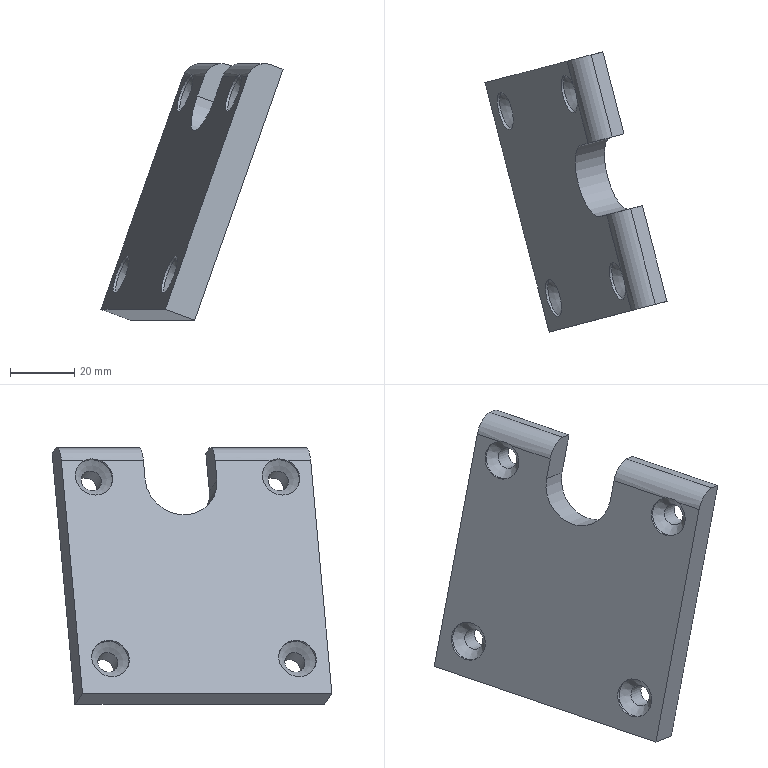Part | STEP file | 车灯-后视镜_id570_x_t | 1 solid | 24 faces | box 56.564 x 86.901 x 79.724 mm | volume 59028 mm3 | cylinder 11 | plane 9 | cone 4 | commonest cylinder face diameters 12 x6 6.5 x4 23 x1
STEP:
#1=CARTESIAN_POINT('',(-178.814,15.991,96.986));
#2=VERTEX_POINT('',#1);
#3=CARTESIAN_POINT('',(-176.662,16.547,103.094));
#4=VERTEX_POINT('',#3);
#5=CARTESIAN_POINT('',(-198.851,10.825,40.135));
#6=DIRECTION('',(0.3312,0.0854,0.9397));
#7=VECTOR('',#6,1.);
#8=LINE('',#5,#7);
#9=EDGE_CURVE('',#2,#4,#8,.T.);
#10=ORIENTED_EDGE('',*,*,#9,.T.);
#11=CARTESIAN_POINT('',(-169.215,18.467,106.68));
#12=VERTEX_POINT('',#11);
#13=CARTESIAN_POINT('',(-171.202,17.954,101.042));
#14=DIRECTION('',(-0.2497,0.9683,0.));
#15=DIRECTION('',(0.9683,0.2497,0.));
#16=AXIS2_PLACEMENT_3D('',#13,#14,#15);
#17=CIRCLE('',#16,6.);
#18=EDGE_CURVE('',#4,#12,#17,.T.);
#19=ORIENTED_EDGE('',*,*,#18,.T.);
#20=CARTESIAN_POINT('',(-165.575,19.405,105.312));
#21=VERTEX_POINT('',#20);
#22=CARTESIAN_POINT('',(-174.674,17.059,108.732));
#23=DIRECTION('',(0.9099,0.2346,-0.342));
#24=VECTOR('',#23,1.);
#25=LINE('',#22,#24);
#26=EDGE_CURVE('',#12,#21,#25,.T.);
#27=ORIENTED_EDGE('',*,*,#26,.T.);
#28=CARTESIAN_POINT('',(-169.715,18.338,93.566));
#29=VERTEX_POINT('',#28);
#30=CARTESIAN_POINT('',(-189.752,13.171,36.714));
#31=DIRECTION('',(0.3312,0.0854,0.9397));
#32=VECTOR('',#31,1.);
#33=LINE('',#30,#32);
#34=EDGE_CURVE('',#29,#21,#33,.T.);
#35=ORIENTED_EDGE('',*,*,#34,.F.);
#36=CARTESIAN_POINT('',(-157.987,21.362,89.158));
#37=DIRECTION('',(-0.9099,-0.2346,0.342));
#38=VECTOR('',#37,1.);
#39=LINE('',#36,#38);
#40=EDGE_CURVE('',#29,#2,#39,.T.);
#41=ORIENTED_EDGE('',*,*,#40,.T.);
#42=EDGE_LOOP('',(#10,#19,#27,#35,#41));
#43=FACE_OUTER_BOUND('',#42,.T.);
#44=CARTESIAN_POINT('',(-155.457,22.015,96.332));
#45=DIRECTION('',(0.2497,-0.9683,0.));
#46=DIRECTION('',(0.9683,0.2497,0.));
#47=AXIS2_PLACEMENT_3D('',#44,#45,#46);
#48=PLANE('',#47);
#49=ADVANCED_FACE('',(#43),#48,.F.);
#50=CARTESIAN_POINT('',(-161.554,-11.242,106.68));
#51=VERTEX_POINT('',#50);
#52=CARTESIAN_POINT('',(-157.914,-10.303,105.312));
#53=VERTEX_POINT('',#52);
#54=CARTESIAN_POINT('',(-167.013,-12.65,108.732));
#55=DIRECTION('',(0.9099,0.2346,-0.342));
#56=VECTOR('',#55,1.);
#57=LINE('',#54,#56);
#58=EDGE_CURVE('',#51,#53,#57,.T.);
#59=ORIENTED_EDGE('',*,*,#58,.F.);
#60=CARTESIAN_POINT('',(-169.001,-13.162,103.094));
#61=VERTEX_POINT('',#60);
#62=CARTESIAN_POINT('',(-163.541,-11.754,101.042));
#63=DIRECTION('',(0.2497,-0.9683,0.));
#64=DIRECTION('',(0.9683,0.2497,0.));
#65=AXIS2_PLACEMENT_3D('',#62,#63,#64);
#66=CIRCLE('',#65,6.);
#67=EDGE_CURVE('',#51,#61,#66,.T.);
#68=ORIENTED_EDGE('',*,*,#67,.T.);
#69=CARTESIAN_POINT('',(-194.502,-19.738,30.738));
#70=VERTEX_POINT('',#69);
#71=CARTESIAN_POINT('',(-178.886,-15.711,75.045));
#72=DIRECTION('',(-0.3312,-0.0854,-0.9397));
#73=VECTOR('',#72,1.);
#74=LINE('',#71,#73);
#75=EDGE_CURVE('',#61,#70,#74,.T.);
#76=ORIENTED_EDGE('',*,*,#75,.T.);
#77=CARTESIAN_POINT('',(-185.403,-17.392,27.318));
#78=VERTEX_POINT('',#77);
#79=CARTESIAN_POINT('',(-194.502,-19.738,30.738));
#80=DIRECTION('',(0.9099,0.2346,-0.342));
#81=VECTOR('',#80,1.);
#82=LINE('',#79,#81);
#83=EDGE_CURVE('',#70,#78,#82,.T.);
#84=ORIENTED_EDGE('',*,*,#83,.T.);
#85=CARTESIAN_POINT('',(-169.787,-13.365,71.625));
#86=DIRECTION('',(-0.3312,-0.0854,-0.9397));
#87=VECTOR('',#86,1.);
#88=LINE('',#85,#87);
#89=EDGE_CURVE('',#53,#78,#88,.T.);
#90=ORIENTED_EDGE('',*,*,#89,.F.);
#91=EDGE_LOOP('',(#59,#68,#76,#84,#90));
#92=FACE_OUTER_BOUND('',#91,.T.);
#93=CARTESIAN_POINT('',(-178.886,-15.711,75.045));
#94=DIRECTION('',(0.2497,-0.9683,0.));
#95=DIRECTION('',(0.9683,0.2497,0.));
#96=AXIS2_PLACEMENT_3D('',#93,#94,#95);
#97=PLANE('',#96);
#98=ADVANCED_FACE('',(#92),#97,.T.);
#99=CARTESIAN_POINT('',(-191.079,-9.073,47.161));
#100=VERTEX_POINT('',#99);
#101=CARTESIAN_POINT('',(-193.19,-9.073,41.544));
#102=DIRECTION('',(0.9099,0.2346,-0.342));
#103=DIRECTION('',(0.3518,0.,0.9361));
#104=AXIS2_PLACEMENT_3D('',#101,#102,#103);
#105=CIRCLE('',#104,6.);
#106=EDGE_CURVE('',#100,#100,#105,.T.);
#107=ORIENTED_EDGE('',*,*,#106,.T.);
#108=EDGE_LOOP('',(#107));
#109=FACE_BOUND('',#108,.T.);
#110=CARTESIAN_POINT('',(-206.061,49.027,47.161));
#111=VERTEX_POINT('',#110);
#112=CARTESIAN_POINT('',(-208.172,49.027,41.544));
#113=DIRECTION('',(0.9099,0.2346,-0.342));
#114=DIRECTION('',(0.3518,0.,0.9361));
#115=AXIS2_PLACEMENT_3D('',#112,#113,#114);
#116=CIRCLE('',#115,6.);
#117=EDGE_CURVE('',#111,#111,#116,.T.);
#118=ORIENTED_EDGE('',*,*,#117,.T.);
#119=EDGE_LOOP('',(#118));
#120=FACE_BOUND('',#119,.T.);
#121=CARTESIAN_POINT('',(-184.557,38.263,96.986));
#122=VERTEX_POINT('',#121);
#123=CARTESIAN_POINT('',(-182.405,38.818,103.094));
#124=VERTEX_POINT('',#123);
#125=CARTESIAN_POINT('',(-204.594,33.096,40.135));
#126=DIRECTION('',(0.3312,0.0854,0.9397));
#127=VECTOR('',#126,1.);
#128=LINE('',#125,#127);
#129=EDGE_CURVE('',#122,#124,#128,.T.);
#130=ORIENTED_EDGE('',*,*,#129,.T.);
#131=CARTESIAN_POINT('',(-185.881,52.298,103.094));
#132=VERTEX_POINT('',#131);
#133=CARTESIAN_POINT('',(-178.93,25.345,103.094));
#134=DIRECTION('',(-0.2497,0.9683,0.));
#135=VECTOR('',#134,1.);
#136=LINE('',#133,#135);
#137=EDGE_CURVE('',#124,#132,#136,.T.);
#138=ORIENTED_EDGE('',*,*,#137,.T.);
#139=CARTESIAN_POINT('',(-187.078,56.942,103.094));
#140=VERTEX_POINT('',#139);
#141=CARTESIAN_POINT('',(-188.301,54.151,97.926));
#142=DIRECTION('',(0.9099,0.2346,-0.342));
#143=DIRECTION('',(0.3518,0.,0.9361));
#144=AXIS2_PLACEMENT_3D('',#141,#142,#143);
#145=CIRCLE('',#144,6.);
#146=EDGE_CURVE('',#132,#140,#145,.T.);
#147=ORIENTED_EDGE('',*,*,#146,.T.);
#148=CARTESIAN_POINT('',(-188.976,64.304,103.094));
#149=VERTEX_POINT('',#148);
#150=CARTESIAN_POINT('',(-178.93,25.345,103.094));
#151=DIRECTION('',(-0.2497,0.9683,0.));
#152=VECTOR('',#151,1.);
#153=LINE('',#150,#152);
#154=EDGE_CURVE('',#140,#149,#153,.T.);
#155=ORIENTED_EDGE('',*,*,#154,.T.);
#156=CARTESIAN_POINT('',(-214.478,57.728,30.738));
#157=VERTEX_POINT('',#156);
#158=CARTESIAN_POINT('',(-198.862,61.754,75.045));
#159=DIRECTION('',(0.3312,0.0854,0.9397));
#160=VECTOR('',#159,1.);
#161=LINE('',#158,#160);
#162=EDGE_CURVE('',#157,#149,#161,.T.);
#163=ORIENTED_EDGE('',*,*,#162,.F.);
#164=CARTESIAN_POINT('',(-204.432,18.769,30.738));
#165=DIRECTION('',(-0.2497,0.9683,0.));
#166=VECTOR('',#165,1.);
#167=LINE('',#164,#166);
#168=EDGE_CURVE('',#70,#157,#167,.T.);
#169=ORIENTED_EDGE('',*,*,#168,.F.);
#170=ORIENTED_EDGE('',*,*,#75,.F.);
#171=CARTESIAN_POINT('',(-170.899,-5.801,103.094));
#172=VERTEX_POINT('',#171);
#173=CARTESIAN_POINT('',(-178.93,25.345,103.094));
#174=DIRECTION('',(-0.2497,0.9683,0.));
#175=VECTOR('',#174,1.);
#176=LINE('',#173,#175);
#177=EDGE_CURVE('',#61,#172,#176,.T.);
#178=ORIENTED_EDGE('',*,*,#177,.T.);
#179=CARTESIAN_POINT('',(-172.096,-1.157,103.094));
#180=VERTEX_POINT('',#179);
#181=CARTESIAN_POINT('',(-173.319,-3.949,97.926));
#182=DIRECTION('',(0.9099,0.2346,-0.342));
#183=DIRECTION('',(0.3518,0.,0.9361));
#184=AXIS2_PLACEMENT_3D('',#181,#182,#183);
#185=CIRCLE('',#184,6.);
#186=EDGE_CURVE('',#172,#180,#185,.T.);
#187=ORIENTED_EDGE('',*,*,#186,.T.);
#188=CARTESIAN_POINT('',(-178.93,25.345,103.094));
#189=DIRECTION('',(-0.2497,0.9683,0.));
#190=VECTOR('',#189,1.);
#191=LINE('',#188,#190);
#192=EDGE_CURVE('',#180,#4,#191,.T.);
#193=ORIENTED_EDGE('',*,*,#192,.T.);
#194=ORIENTED_EDGE('',*,*,#9,.F.);
#195=CARTESIAN_POINT('',(-181.686,27.127,96.986));
#196=DIRECTION('',(0.9099,0.2346,-0.342));
#197=DIRECTION('',(0.3518,0.,0.9361));
#198=AXIS2_PLACEMENT_3D('',#195,#196,#197);
#199=CIRCLE('',#198,11.5);
#200=EDGE_CURVE('',#2,#122,#199,.T.);
#201=ORIENTED_EDGE('',*,*,#200,.T.);
#202=EDGE_LOOP('',(#130,#138,#147,#155,#163,#169,#170,#178,#187,#193,#194,#201));
#203=FACE_BOUND('',#202,.T.);
#204=CARTESIAN_POINT('',(-201.12,19.623,40.135));
#205=DIRECTION('',(-0.9099,-0.2346,0.342));
#206=DIRECTION('',(0.3518,0.,0.9361));
#207=AXIS2_PLACEMENT_3D('',#204,#205,#206);
#208=PLANE('',#207);
#209=ADVANCED_FACE('',(#109,#120,#203),#208,.T.);
#210=CARTESIAN_POINT('',(-182.948,-6.726,41.166));
#211=VERTEX_POINT('',#210);
#212=CARTESIAN_POINT('',(-184.091,-6.726,38.124));
#213=DIRECTION('',(0.9099,0.2346,-0.342));
#214=DIRECTION('',(0.3518,0.,0.9361));
#215=AXIS2_PLACEMENT_3D('',#212,#213,#214);
#216=CIRCLE('',#215,3.25);
#217=EDGE_CURVE('',#211,#211,#216,.T.);
#218=ORIENTED_EDGE('',*,*,#217,.F.);
#219=EDGE_LOOP('',(#218));
#220=FACE_BOUND('',#219,.T.);
#221=CARTESIAN_POINT('',(-197.929,51.373,41.166));
#222=VERTEX_POINT('',#221);
#223=CARTESIAN_POINT('',(-199.073,51.373,38.124));
#224=DIRECTION('',(0.9099,0.2346,-0.342));
#225=DIRECTION('',(0.3518,0.,0.9361));
#226=AXIS2_PLACEMENT_3D('',#223,#224,#225);
#227=CIRCLE('',#226,3.25);
#228=EDGE_CURVE('',#222,#222,#227,.T.);
#229=ORIENTED_EDGE('',*,*,#228,.F.);
#230=EDGE_LOOP('',(#229));
#231=FACE_BOUND('',#230,.T.);
#232=CARTESIAN_POINT('',(-178.058,56.497,97.548));
#233=VERTEX_POINT('',#232);
#234=CARTESIAN_POINT('',(-179.202,56.497,94.506));
#235=DIRECTION('',(0.9099,0.2346,-0.342));
#236=DIRECTION('',(0.3518,0.,0.9361));
#237=AXIS2_PLACEMENT_3D('',#234,#235,#236);
#238=CIRCLE('',#237,3.25);
#239=EDGE_CURVE('',#233,#233,#238,.T.);
#240=ORIENTED_EDGE('',*,*,#239,.F.);
#241=EDGE_LOOP('',(#240));
#242=FACE_BOUND('',#241,.T.);
#243=CARTESIAN_POINT('',(-163.076,-1.602,97.548));
#244=VERTEX_POINT('',#243);
#245=CARTESIAN_POINT('',(-164.22,-1.602,94.506));
#246=DIRECTION('',(0.9099,0.2346,-0.342));
#247=DIRECTION('',(0.3518,0.,0.9361));
#248=AXIS2_PLACEMENT_3D('',#245,#246,#247);
#249=CIRCLE('',#248,3.25);
#250=EDGE_CURVE('',#244,#244,#249,.T.);
#251=ORIENTED_EDGE('',*,*,#250,.F.);
#252=EDGE_LOOP('',(#251));
#253=FACE_BOUND('',#252,.T.);
#254=CARTESIAN_POINT('',(-205.379,60.074,27.318));
#255=VERTEX_POINT('',#254);
#256=CARTESIAN_POINT('',(-195.332,21.116,27.318));
#257=DIRECTION('',(-0.2497,0.9683,0.));
#258=VECTOR('',#257,1.);
#259=LINE('',#256,#258);
#260=EDGE_CURVE('',#78,#255,#259,.T.);
#261=ORIENTED_EDGE('',*,*,#260,.T.);
#262=CARTESIAN_POINT('',(-177.89,67.162,105.312));
#263=VERTEX_POINT('',#262);
#264=CARTESIAN_POINT('',(-189.763,64.101,71.625));
#265=DIRECTION('',(0.3312,0.0854,0.9397));
#266=VECTOR('',#265,1.);
#267=LINE('',#264,#266);
#268=EDGE_CURVE('',#255,#263,#267,.T.);
#269=ORIENTED_EDGE('',*,*,#268,.T.);
#270=CARTESIAN_POINT('',(-171.318,41.677,105.312));
#271=VERTEX_POINT('',#270);
#272=CARTESIAN_POINT('',(-167.844,28.204,105.312));
#273=DIRECTION('',(0.2497,-0.9683,0.));
#274=VECTOR('',#273,1.);
#275=LINE('',#272,#274);
#276=EDGE_CURVE('',#263,#271,#275,.T.);
#277=ORIENTED_EDGE('',*,*,#276,.T.);
#278=CARTESIAN_POINT('',(-175.458,40.609,93.566));
#279=VERTEX_POINT('',#278);
#280=CARTESIAN_POINT('',(-195.495,35.442,36.714));
#281=DIRECTION('',(0.3312,0.0854,0.9397));
#282=VECTOR('',#281,1.);
#283=LINE('',#280,#282);
#284=EDGE_CURVE('',#279,#271,#283,.T.);
#285=ORIENTED_EDGE('',*,*,#284,.F.);
#286=CARTESIAN_POINT('',(-172.586,29.474,93.566));
#287=DIRECTION('',(-0.9099,-0.2346,0.342));
#288=DIRECTION('',(0.3518,0.,0.9361));
#289=AXIS2_PLACEMENT_3D('',#286,#287,#288);
#290=CIRCLE('',#289,11.5);
#291=EDGE_CURVE('',#279,#29,#290,.T.);
#292=ORIENTED_EDGE('',*,*,#291,.T.);
#293=ORIENTED_EDGE('',*,*,#34,.T.);
#294=CARTESIAN_POINT('',(-167.844,28.204,105.312));
#295=DIRECTION('',(0.2497,-0.9683,0.));
#296=VECTOR('',#295,1.);
#297=LINE('',#294,#296);
#298=EDGE_CURVE('',#21,#53,#297,.T.);
#299=ORIENTED_EDGE('',*,*,#298,.T.);
#300=ORIENTED_EDGE('',*,*,#89,.T.);
#301=EDGE_LOOP('',(#261,#269,#277,#285,#292,#293,#299,#300));
#302=FACE_BOUND('',#301,.T.);
#303=CARTESIAN_POINT('',(-192.021,21.97,36.714));
#304=DIRECTION('',(-0.9099,-0.2346,0.342));
#305=DIRECTION('',(0.3518,0.,0.9361));
#306=AXIS2_PLACEMENT_3D('',#303,#304,#305);
#307=PLANE('',#306);
#308=ADVANCED_FACE('',(#220,#231,#242,#253,#302),#307,.F.);
#309=ORIENTED_EDGE('',*,*,#168,.T.);
#310=CARTESIAN_POINT('',(-214.478,57.728,30.738));
#311=DIRECTION('',(0.9099,0.2346,-0.342));
#312=VECTOR('',#311,1.);
#313=LINE('',#310,#312);
#314=EDGE_CURVE('',#157,#255,#313,.T.);
#315=ORIENTED_EDGE('',*,*,#314,.T.);
#316=ORIENTED_EDGE('',*,*,#260,.F.);
#317=ORIENTED_EDGE('',*,*,#83,.F.);
#318=EDGE_LOOP('',(#309,#315,#316,#317));
#319=FACE_OUTER_BOUND('',#318,.T.);
#320=CARTESIAN_POINT('',(-204.432,18.769,30.738));
#321=DIRECTION('',(-0.3312,-0.0854,-0.9397));
#322=DIRECTION('',(-0.9431,0.,0.3324));
#323=AXIS2_PLACEMENT_3D('',#320,#321,#322);
#324=PLANE('',#323);
#325=ADVANCED_FACE('',(#319),#324,.T.);
#326=ORIENTED_EDGE('',*,*,#26,.F.);
#327=CARTESIAN_POINT('',(-171.484,27.265,106.68));
#328=DIRECTION('',(0.2497,-0.9683,0.));
#329=VECTOR('',#328,1.);
#330=LINE('',#327,#329);
#331=EDGE_CURVE('',#12,#51,#330,.T.);
#332=ORIENTED_EDGE('',*,*,#331,.T.);
#333=ORIENTED_EDGE('',*,*,#58,.T.);
#334=ORIENTED_EDGE('',*,*,#298,.F.);
#335=EDGE_LOOP('',(#326,#332,#333,#334));
#336=FACE_OUTER_BOUND('',#335,.T.);
#337=CARTESIAN_POINT('',(-176.943,25.858,108.732));
#338=DIRECTION('',(0.3312,0.0854,0.9397));
#339=DIRECTION('',(0.9431,0.,-0.3324));
#340=AXIS2_PLACEMENT_3D('',#337,#338,#339);
#341=PLANE('',#340);
#342=ADVANCED_FACE('',(#336),#341,.T.);
#343=CARTESIAN_POINT('',(-181.53,66.224,106.68));
#344=VERTEX_POINT('',#343);
#345=CARTESIAN_POINT('',(-186.989,64.816,108.732));
#346=DIRECTION('',(0.9099,0.2346,-0.342));
#347=VECTOR('',#346,1.);
#348=LINE('',#345,#347);
#349=EDGE_CURVE('',#344,#263,#348,.T.);
#350=ORIENTED_EDGE('',*,*,#349,.F.);
#351=CARTESIAN_POINT('',(-174.958,40.738,106.68));
#352=VERTEX_POINT('',#351);
#353=CARTESIAN_POINT('',(-171.484,27.265,106.68));
#354=DIRECTION('',(0.2497,-0.9683,0.));
#355=VECTOR('',#354,1.);
#356=LINE('',#353,#355);
#357=EDGE_CURVE('',#344,#352,#356,.T.);
#358=ORIENTED_EDGE('',*,*,#357,.T.);
#359=CARTESIAN_POINT('',(-180.417,39.33,108.732));
#360=DIRECTION('',(0.9099,0.2346,-0.342));
#361=VECTOR('',#360,1.);
#362=LINE('',#359,#361);
#363=EDGE_CURVE('',#352,#271,#362,.T.);
#364=ORIENTED_EDGE('',*,*,#363,.T.);
#365=ORIENTED_EDGE('',*,*,#276,.F.);
#366=EDGE_LOOP('',(#350,#358,#364,#365));
#367=FACE_OUTER_BOUND('',#366,.T.);
#368=CARTESIAN_POINT('',(-176.943,25.858,108.732));
#369=DIRECTION('',(0.3312,0.0854,0.9397));
#370=DIRECTION('',(0.9431,0.,-0.3324));
#371=AXIS2_PLACEMENT_3D('',#368,#369,#370);
#372=PLANE('',#371);
#373=ADVANCED_FACE('',(#367),#372,.T.);
#374=ORIENTED_EDGE('',*,*,#162,.T.);
#375=CARTESIAN_POINT('',(-183.517,65.711,101.042));
#376=DIRECTION('',(-0.2497,0.9683,0.));
#377=DIRECTION('',(-0.9683,-0.2497,0.));
#378=AXIS2_PLACEMENT_3D('',#375,#376,#377);
#379=CIRCLE('',#378,6.);
#380=EDGE_CURVE('',#149,#344,#379,.T.);
#381=ORIENTED_EDGE('',*,*,#380,.T.);
#382=ORIENTED_EDGE('',*,*,#349,.T.);
#383=ORIENTED_EDGE('',*,*,#268,.F.);
#384=ORIENTED_EDGE('',*,*,#314,.F.);
#385=EDGE_LOOP('',(#374,#381,#382,#383,#384));
#386=FACE_OUTER_BOUND('',#385,.T.);
#387=CARTESIAN_POINT('',(-198.862,61.754,75.045));
#388=DIRECTION('',(-0.2497,0.9683,0.));
#389=DIRECTION('',(-0.9683,-0.2497,0.));
#390=AXIS2_PLACEMENT_3D('',#387,#388,#389);
#391=PLANE('',#390);
#392=ADVANCED_FACE('',(#386),#391,.T.);
#393=ORIENTED_EDGE('',*,*,#363,.F.);
#394=CARTESIAN_POINT('',(-176.945,40.226,101.042));
#395=DIRECTION('',(0.2497,-0.9683,0.));
#396=DIRECTION('',(0.9683,0.2497,0.));
#397=AXIS2_PLACEMENT_3D('',#394,#395,#396);
#398=CIRCLE('',#397,6.);
#399=EDGE_CURVE('',#352,#124,#398,.T.);
#400=ORIENTED_EDGE('',*,*,#399,.T.);
#401=ORIENTED_EDGE('',*,*,#129,.F.);
#402=CARTESIAN_POINT('',(-163.73,43.634,89.158));
#403=DIRECTION('',(0.9099,0.2346,-0.342));
#404=VECTOR('',#403,1.);
#405=LINE('',#402,#404);
#406=EDGE_CURVE('',#122,#279,#405,.T.);
#407=ORIENTED_EDGE('',*,*,#406,.T.);
#408=ORIENTED_EDGE('',*,*,#284,.T.);
#409=EDGE_LOOP('',(#393,#400,#401,#407,#408));
#410=FACE_OUTER_BOUND('',#409,.T.);
#411=CARTESIAN_POINT('',(-161.201,44.286,96.332));
#412=DIRECTION('',(0.2497,-0.9683,0.));
#413=DIRECTION('',(0.9683,0.2497,0.));
#414=AXIS2_PLACEMENT_3D('',#411,#412,#413);
#415=PLANE('',#414);
#416=ADVANCED_FACE('',(#410),#415,.T.);
#417=ORIENTED_EDGE('',*,*,#406,.F.);
#418=ORIENTED_EDGE('',*,*,#200,.F.);
#419=ORIENTED_EDGE('',*,*,#40,.F.);
#420=ORIENTED_EDGE('',*,*,#291,.F.);
#421=EDGE_LOOP('',(#417,#418,#419,#420));
#422=FACE_OUTER_BOUND('',#421,.T.);
#423=CARTESIAN_POINT('',(-160.859,32.498,89.158));
#424=DIRECTION('',(-0.9099,-0.2346,0.342));
#425=DIRECTION('',(0.3518,0.,0.9361));
#426=AXIS2_PLACEMENT_3D('',#423,#424,#425);
#427=CYLINDRICAL_SURFACE('',#426,11.5);
#428=ADVANCED_FACE('',(#422),#427,.F.);
#429=CARTESIAN_POINT('',(-170.48,-3.761,103.268));
#430=VERTEX_POINT('',#429);
#431=CARTESIAN_POINT('',(-172.591,-3.761,97.652));
#432=DIRECTION('',(0.9099,0.2346,-0.342));
#433=DIRECTION('',(0.3518,0.,0.9361));
#434=AXIS2_PLACEMENT_3D('',#431,#432,#433);
#435=CIRCLE('',#434,6.);
#436=EDGE_CURVE('',#430,#430,#435,.T.);
#437=ORIENTED_EDGE('',*,*,#436,.T.);
#438=EDGE_LOOP('',(#437));
#439=FACE_BOUND('',#438,.T.);
#440=ORIENTED_EDGE('',*,*,#186,.F.);
#441=CARTESIAN_POINT('',(-170.899,-5.801,103.094));
#442=CARTESIAN_POINT('',(-171.059,-4.273,103.717));
#443=CARTESIAN_POINT('',(-171.497,-2.572,103.717));
#444=CARTESIAN_POINT('',(-172.096,-1.157,103.094));
#445=B_SPLINE_CURVE_WITH_KNOTS('',3,(#441,#442,#443,#444),.UNSPECIFIED.,.F.,.F.,(4,4),(0.,1.),.UNSPECIFIED.);
#446=EDGE_CURVE('',#172,#180,#445,.T.);
#447=ORIENTED_EDGE('',*,*,#446,.T.);
#448=EDGE_LOOP('',(#440,#447));
#449=FACE_BOUND('',#448,.T.);
#450=CARTESIAN_POINT('',(-172.864,-3.831,97.755));
#451=DIRECTION('',(0.9099,0.2346,-0.342));
#452=DIRECTION('',(-0.3518,0.,-0.9361));
#453=AXIS2_PLACEMENT_3D('',#450,#451,#452);
#454=CYLINDRICAL_SURFACE('',#453,6.);
#455=ADVANCED_FACE('',(#439,#449),#454,.F.);
#456=CARTESIAN_POINT('',(-168.945,-3.116,99.754));
#457=VERTEX_POINT('',#456);
#458=CARTESIAN_POINT('',(-170.089,-3.116,96.712));
#459=DIRECTION('',(0.9099,0.2346,-0.342));
#460=DIRECTION('',(0.3518,0.,0.9361));
#461=AXIS2_PLACEMENT_3D('',#458,#459,#460);
#462=CIRCLE('',#461,3.25);
#463=EDGE_CURVE('',#457,#457,#462,.T.);
#464=ORIENTED_EDGE('',*,*,#463,.T.);
#465=EDGE_LOOP('',(#464));
#466=FACE_BOUND('',#465,.T.);
#467=ORIENTED_EDGE('',*,*,#436,.F.);
#468=EDGE_LOOP('',(#467));
#469=FACE_BOUND('',#468,.T.);
#470=CARTESIAN_POINT('',(-172.591,-3.761,97.652));
#471=DIRECTION('',(-0.9099,-0.2346,0.342));
#472=DIRECTION('',(-0.3518,0.,-0.9361));
#473=AXIS2_PLACEMENT_3D('',#470,#471,#472);
#474=CONICAL_SURFACE('',#473,6.,45.);
#475=ADVANCED_FACE('',(#466,#469),#474,.F.);
#476=ORIENTED_EDGE('',*,*,#250,.T.);
#477=EDGE_LOOP('',(#476));
#478=FACE_BOUND('',#477,.T.);
#479=ORIENTED_EDGE('',*,*,#463,.F.);
#480=EDGE_LOOP('',(#479));
#481=FACE_BOUND('',#480,.T.);
#482=CARTESIAN_POINT('',(-169.861,-3.057,96.626));
#483=DIRECTION('',(0.9099,0.2346,-0.342));
#484=DIRECTION('',(-0.3518,0.,-0.9361));
#485=AXIS2_PLACEMENT_3D('',#482,#483,#484);
#486=CYLINDRICAL_SURFACE('',#485,3.25);
#487=ADVANCED_FACE('',(#478,#481),#486,.F.);
#488=CARTESIAN_POINT('',(-185.462,54.338,103.268));
#489=VERTEX_POINT('',#488);
#490=CARTESIAN_POINT('',(-187.573,54.338,97.652));
#491=DIRECTION('',(0.9099,0.2346,-0.342));
#492=DIRECTION('',(0.3518,0.,0.9361));
#493=AXIS2_PLACEMENT_3D('',#490,#491,#492);
#494=CIRCLE('',#493,6.);
#495=EDGE_CURVE('',#489,#489,#494,.T.);
#496=ORIENTED_EDGE('',*,*,#495,.T.);
#497=EDGE_LOOP('',(#496));
#498=FACE_BOUND('',#497,.T.);
#499=ORIENTED_EDGE('',*,*,#146,.F.);
#500=CARTESIAN_POINT('',(-185.881,52.298,103.094));
#501=CARTESIAN_POINT('',(-186.041,53.827,103.717));
#502=CARTESIAN_POINT('',(-186.479,55.527,103.717));
#503=CARTESIAN_POINT('',(-187.078,56.942,103.094));
#504=B_SPLINE_CURVE_WITH_KNOTS('',3,(#500,#501,#502,#503),.UNSPECIFIED.,.F.,.F.,(4,4),(0.,1.),.UNSPECIFIED.);
#505=EDGE_CURVE('',#132,#140,#504,.T.);
#506=ORIENTED_EDGE('',*,*,#505,.T.);
#507=EDGE_LOOP('',(#499,#506));
#508=FACE_BOUND('',#507,.T.);
#509=CARTESIAN_POINT('',(-187.846,54.268,97.755));
#510=DIRECTION('',(0.9099,0.2346,-0.342));
#511=DIRECTION('',(-0.3518,0.,-0.9361));
#512=AXIS2_PLACEMENT_3D('',#509,#510,#511);
#513=CYLINDRICAL_SURFACE('',#512,6.);
#514=ADVANCED_FACE('',(#498,#508),#513,.F.);
#515=CARTESIAN_POINT('',(-183.927,54.984,99.754));
#516=VERTEX_POINT('',#515);
#517=CARTESIAN_POINT('',(-185.071,54.984,96.712));
#518=DIRECTION('',(0.9099,0.2346,-0.342));
#519=DIRECTION('',(0.3518,0.,0.9361));
#520=AXIS2_PLACEMENT_3D('',#517,#518,#519);
#521=CIRCLE('',#520,3.25);
#522=EDGE_CURVE('',#516,#516,#521,.T.);
#523=ORIENTED_EDGE('',*,*,#522,.T.);
#524=EDGE_LOOP('',(#523));
#525=FACE_BOUND('',#524,.T.);
#526=ORIENTED_EDGE('',*,*,#495,.F.);
#527=EDGE_LOOP('',(#526));
#528=FACE_BOUND('',#527,.T.);
#529=CARTESIAN_POINT('',(-187.573,54.338,97.652));
#530=DIRECTION('',(-0.9099,-0.2346,0.342));
#531=DIRECTION('',(-0.3518,0.,-0.9361));
#532=AXIS2_PLACEMENT_3D('',#529,#530,#531);
#533=CONICAL_SURFACE('',#532,6.,45.);
#534=ADVANCED_FACE('',(#525,#528),#533,.F.);
#535=ORIENTED_EDGE('',*,*,#239,.T.);
#536=EDGE_LOOP('',(#535));
#537=FACE_BOUND('',#536,.T.);
#538=ORIENTED_EDGE('',*,*,#522,.F.);
#539=EDGE_LOOP('',(#538));
#540=FACE_BOUND('',#539,.T.);
#541=CARTESIAN_POINT('',(-184.843,55.042,96.626));
#542=DIRECTION('',(0.9099,0.2346,-0.342));
#543=DIRECTION('',(-0.3518,0.,-0.9361));
#544=AXIS2_PLACEMENT_3D('',#541,#542,#543);
#545=CYLINDRICAL_SURFACE('',#544,3.25);
#546=ADVANCED_FACE('',(#537,#540),#545,.F.);
#547=CARTESIAN_POINT('',(-205.333,49.214,46.887));
#548=VERTEX_POINT('',#547);
#549=CARTESIAN_POINT('',(-207.444,49.214,41.271));
#550=DIRECTION('',(0.9099,0.2346,-0.342));
#551=DIRECTION('',(0.3518,0.,0.9361));
#552=AXIS2_PLACEMENT_3D('',#549,#550,#551);
#553=CIRCLE('',#552,6.);
#554=EDGE_CURVE('',#548,#548,#553,.T.);
#555=ORIENTED_EDGE('',*,*,#554,.T.);
#556=EDGE_LOOP('',(#555));
#557=FACE_BOUND('',#556,.T.);
#558=ORIENTED_EDGE('',*,*,#117,.F.);
#559=EDGE_LOOP('',(#558));
#560=FACE_BOUND('',#559,.T.);
#561=CARTESIAN_POINT('',(-207.717,49.144,41.373));
#562=DIRECTION('',(0.9099,0.2346,-0.342));
#563=DIRECTION('',(-0.3518,0.,-0.9361));
#564=AXIS2_PLACEMENT_3D('',#561,#562,#563);
#565=CYLINDRICAL_SURFACE('',#564,6.);
#566=ADVANCED_FACE('',(#557,#560),#565,.F.);
#567=CARTESIAN_POINT('',(-203.798,49.859,43.372));
#568=VERTEX_POINT('',#567);
#569=CARTESIAN_POINT('',(-204.942,49.859,40.33));
#570=DIRECTION('',(0.9099,0.2346,-0.342));
#571=DIRECTION('',(0.3518,0.,0.9361));
#572=AXIS2_PLACEMENT_3D('',#569,#570,#571);
#573=CIRCLE('',#572,3.25);
#574=EDGE_CURVE('',#568,#568,#573,.T.);
#575=ORIENTED_EDGE('',*,*,#574,.T.);
#576=EDGE_LOOP('',(#575));
#577=FACE_BOUND('',#576,.T.);
#578=ORIENTED_EDGE('',*,*,#554,.F.);
#579=EDGE_LOOP('',(#578));
#580=FACE_BOUND('',#579,.T.);
#581=CARTESIAN_POINT('',(-207.444,49.214,41.271));
#582=DIRECTION('',(-0.9099,-0.2346,0.342));
#583=DIRECTION('',(-0.3518,0.,-0.9361));
#584=AXIS2_PLACEMENT_3D('',#581,#582,#583);
#585=CONICAL_SURFACE('',#584,6.,45.);
#586=ADVANCED_FACE('',(#577,#580),#585,.F.);
#587=ORIENTED_EDGE('',*,*,#228,.T.);
#588=EDGE_LOOP('',(#587));
#589=FACE_BOUND('',#588,.T.);
#590=ORIENTED_EDGE('',*,*,#574,.F.);
#591=EDGE_LOOP('',(#590));
#592=FACE_BOUND('',#591,.T.);
#593=CARTESIAN_POINT('',(-204.714,49.918,40.245));
#594=DIRECTION('',(0.9099,0.2346,-0.342));
#595=DIRECTION('',(-0.3518,0.,-0.9361));
#596=AXIS2_PLACEMENT_3D('',#593,#594,#595);
#597=CYLINDRICAL_SURFACE('',#596,3.25);
#598=ADVANCED_FACE('',(#589,#592),#597,.F.);
#599=CARTESIAN_POINT('',(-190.351,-8.885,46.887));
#600=VERTEX_POINT('',#599);
#601=CARTESIAN_POINT('',(-192.462,-8.885,41.271));
#602=DIRECTION('',(0.9099,0.2346,-0.342));
#603=DIRECTION('',(0.3518,0.,0.9361));
#604=AXIS2_PLACEMENT_3D('',#601,#602,#603);
#605=CIRCLE('',#604,6.);
#606=EDGE_CURVE('',#600,#600,#605,.T.);
#607=ORIENTED_EDGE('',*,*,#606,.T.);
#608=EDGE_LOOP('',(#607));
#609=FACE_BOUND('',#608,.T.);
#610=ORIENTED_EDGE('',*,*,#106,.F.);
#611=EDGE_LOOP('',(#610));
#612=FACE_BOUND('',#611,.T.);
#613=CARTESIAN_POINT('',(-192.735,-8.956,41.373));
#614=DIRECTION('',(0.9099,0.2346,-0.342));
#615=DIRECTION('',(-0.3518,0.,-0.9361));
#616=AXIS2_PLACEMENT_3D('',#613,#614,#615);
#617=CYLINDRICAL_SURFACE('',#616,6.);
#618=ADVANCED_FACE('',(#609,#612),#617,.F.);
#619=CARTESIAN_POINT('',(-188.817,-8.24,43.372));
#620=VERTEX_POINT('',#619);
#621=CARTESIAN_POINT('',(-189.96,-8.24,40.33));
#622=DIRECTION('',(0.9099,0.2346,-0.342));
#623=DIRECTION('',(0.3518,0.,0.9361));
#624=AXIS2_PLACEMENT_3D('',#621,#622,#623);
#625=CIRCLE('',#624,3.25);
#626=EDGE_CURVE('',#620,#620,#625,.T.);
#627=ORIENTED_EDGE('',*,*,#626,.T.);
#628=EDGE_LOOP('',(#627));
#629=FACE_BOUND('',#628,.T.);
#630=ORIENTED_EDGE('',*,*,#606,.F.);
#631=EDGE_LOOP('',(#630));
#632=FACE_BOUND('',#631,.T.);
#633=CARTESIAN_POINT('',(-192.462,-8.885,41.271));
#634=DIRECTION('',(-0.9099,-0.2346,0.342));
#635=DIRECTION('',(-0.3518,0.,-0.9361));
#636=AXIS2_PLACEMENT_3D('',#633,#634,#635);
#637=CONICAL_SURFACE('',#636,6.,45.);
#638=ADVANCED_FACE('',(#629,#632),#637,.F.);
#639=ORIENTED_EDGE('',*,*,#217,.T.);
#640=EDGE_LOOP('',(#639));
#641=FACE_BOUND('',#640,.T.);
#642=ORIENTED_EDGE('',*,*,#626,.F.);
#643=EDGE_LOOP('',(#642));
#644=FACE_BOUND('',#643,.T.);
#645=CARTESIAN_POINT('',(-189.733,-8.181,40.245));
#646=DIRECTION('',(0.9099,0.2346,-0.342));
#647=DIRECTION('',(-0.3518,0.,-0.9361));
#648=AXIS2_PLACEMENT_3D('',#645,#646,#647);
#649=CYLINDRICAL_SURFACE('',#648,3.25);
#650=ADVANCED_FACE('',(#641,#644),#649,.F.);
#651=ORIENTED_EDGE('',*,*,#399,.F.);
#652=ORIENTED_EDGE('',*,*,#357,.F.);
#653=ORIENTED_EDGE('',*,*,#380,.F.);
#654=ORIENTED_EDGE('',*,*,#154,.F.);
#655=ORIENTED_EDGE('',*,*,#505,.F.);
#656=ORIENTED_EDGE('',*,*,#137,.F.);
#657=EDGE_LOOP('',(#651,#652,#653,#654,#655,#656));
#658=FACE_OUTER_BOUND('',#657,.T.);
#659=CARTESIAN_POINT('',(-173.471,26.753,101.042));
#660=DIRECTION('',(-0.2497,0.9683,0.));
#661=DIRECTION('',(-0.9683,-0.2497,0.));
#662=AXIS2_PLACEMENT_3D('',#659,#660,#661);
#663=CYLINDRICAL_SURFACE('',#662,6.);
#664=ADVANCED_FACE('',(#658),#663,.T.);
#665=ORIENTED_EDGE('',*,*,#67,.F.);
#666=ORIENTED_EDGE('',*,*,#331,.F.);
#667=ORIENTED_EDGE('',*,*,#18,.F.);
#668=ORIENTED_EDGE('',*,*,#192,.F.);
#669=ORIENTED_EDGE('',*,*,#446,.F.);
#670=ORIENTED_EDGE('',*,*,#177,.F.);
#671=EDGE_LOOP('',(#665,#666,#667,#668,#669,#670));
#672=FACE_OUTER_BOUND('',#671,.T.);
#673=CARTESIAN_POINT('',(-173.471,26.753,101.042));
#674=DIRECTION('',(-0.2497,0.9683,0.));
#675=DIRECTION('',(-0.9683,-0.2497,0.));
#676=AXIS2_PLACEMENT_3D('',#673,#674,#675);
#677=CYLINDRICAL_SURFACE('',#676,6.);
#678=ADVANCED_FACE('',(#672),#677,.T.);
#679=CLOSED_SHELL('',(#49,#98,#209,#308,#325,#342,#373,#392,#416,#428,#455,#475,#487,#514,#534,#546,#566,#586,#598,#618,#638,#650,#664,#678));
#680=MANIFOLD_SOLID_BREP('',#679);
#681=(LENGTH_UNIT()NAMED_UNIT(*)SI_UNIT(.MILLI.,.METRE.));
#682=UNCERTAINTY_MEASURE_WITH_UNIT(LENGTH_MEASURE(0.0508),#681,'','');
#683=(NAMED_UNIT(*)PLANE_ANGLE_UNIT()SI_UNIT($,.RADIAN.));
#684=PLANE_ANGLE_MEASURE_WITH_UNIT(PLANE_ANGLE_MEASURE(0.01745),#683);
#685=DIMENSIONAL_EXPONENTS(0.,0.,0.,0.,0.,0.,0.);
#686=(CONVERSION_BASED_UNIT('DEGREE',#684)NAMED_UNIT(#685)PLANE_ANGLE_UNIT());
#687=(NAMED_UNIT(*)SI_UNIT($,.STERADIAN.)SOLID_ANGLE_UNIT());
#688=(GEOMETRIC_REPRESENTATION_CONTEXT(3)GLOBAL_UNCERTAINTY_ASSIGNED_CONTEXT((#682))GLOBAL_UNIT_ASSIGNED_CONTEXT((#681,#686,#687))REPRESENTATION_CONTEXT('',''));
#689=ADVANCED_BREP_SHAPE_REPRESENTATION('',(#680),#688);